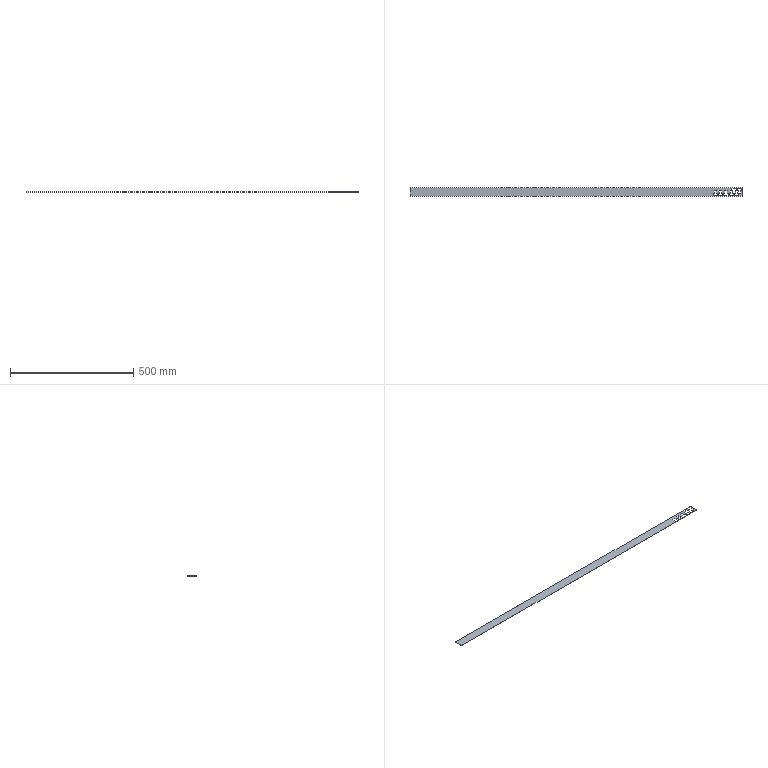Part | Creo | features DATUM PLANE 3, CURVE 2, PROTRUSION 2, COORDINATE SYSTEM 1 | 1 solid | 118 faces | box 1347 x 36.003 x 0.5 mm | volume 23317 mm3 | plane 62 | cylinder 56 | commonest cylinder face diameters 0.75 x56